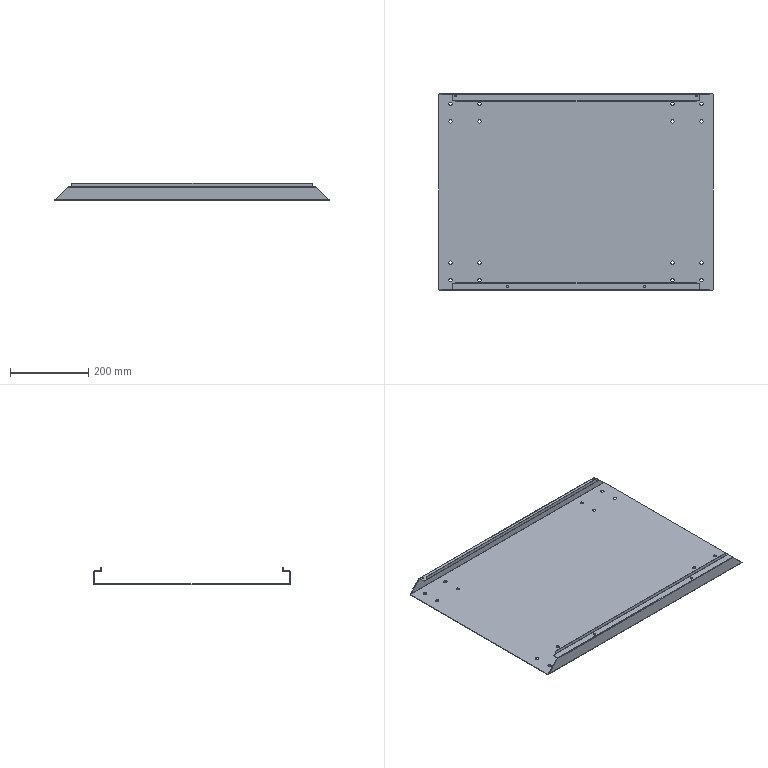Part | SolidWorks | features EdgeFlange 3, ICE 2, FlatPattern 1, MirrorPattern 1, SMBaseFlange 1, SheetMetal 1 | 1 solid | 100 faces | box 700 x 500 x 43.5 mm | volume 635964 mm3 | plane 54 | cylinder 46 | commonest cylinder face diameters 8.5 x32 3 x6 4.5 x4 6.5 x4